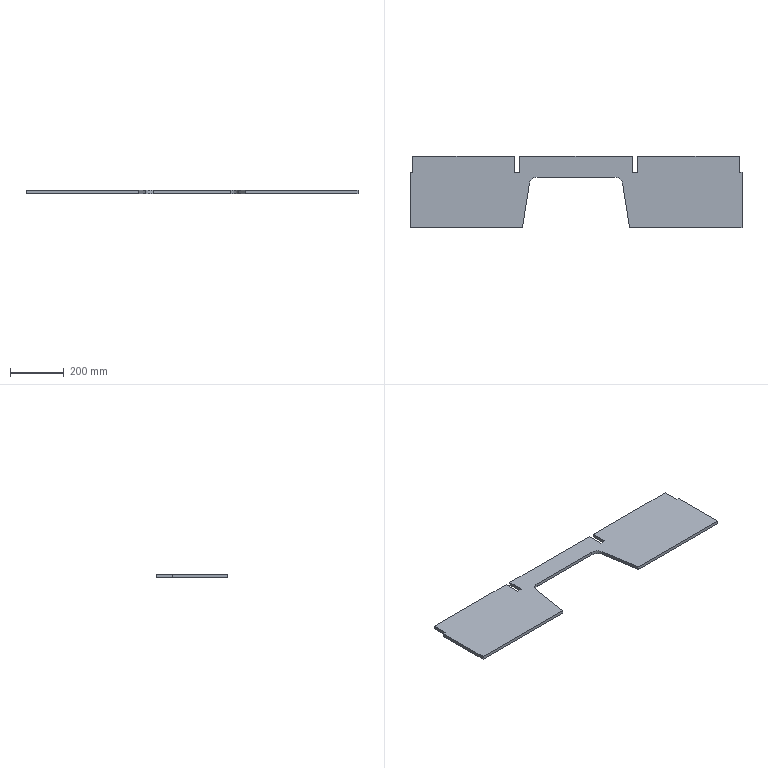Part | SolidWorks | features Extrusion 1 | 1 solid | 24 faces | box 1240 x 268 x 12 mm | volume 3104432 mm3 | plane 22 | cylinder 2 | commonest cylinder face diameters 60 x2
STEP:
#1=CARTESIAN_POINT('',(0.,208.,0.));
#2=VERTEX_POINT('',#1);
#3=CARTESIAN_POINT('',(0.,0.,0.));
#4=VERTEX_POINT('',#3);
#5=CARTESIAN_POINT('',(0.,0.,0.));
#6=DIRECTION('',(0.,-1.,0.));
#7=VECTOR('',#6,1000.);
#8=LINE('',#5,#7);
#9=EDGE_CURVE('',#2,#4,#8,.T.);
#10=ORIENTED_EDGE('',*,*,#9,.T.);
#11=CARTESIAN_POINT('',(0.,0.,12.));
#12=VERTEX_POINT('',#11);
#13=CARTESIAN_POINT('',(0.,0.,12.));
#14=DIRECTION('',(0.,0.,-1.));
#15=VECTOR('',#14,1000.);
#16=LINE('',#13,#15);
#17=EDGE_CURVE('',#12,#4,#16,.T.);
#18=ORIENTED_EDGE('',*,*,#17,.F.);
#19=CARTESIAN_POINT('',(0.,208.,12.));
#20=VERTEX_POINT('',#19);
#21=CARTESIAN_POINT('',(0.,0.,12.));
#22=DIRECTION('',(0.,-1.,0.));
#23=VECTOR('',#22,1000.);
#24=LINE('',#21,#23);
#25=EDGE_CURVE('',#20,#12,#24,.T.);
#26=ORIENTED_EDGE('',*,*,#25,.F.);
#27=CARTESIAN_POINT('',(0.,208.,12.));
#28=DIRECTION('',(0.,0.,-1.));
#29=VECTOR('',#28,1000.);
#30=LINE('',#27,#29);
#31=EDGE_CURVE('',#20,#2,#30,.T.);
#32=ORIENTED_EDGE('',*,*,#31,.T.);
#33=EDGE_LOOP('',(#10,#18,#26,#32));
#34=FACE_OUTER_BOUND('',#33,.T.);
#35=CARTESIAN_POINT('',(0.,0.,12.));
#36=DIRECTION('',(1.,0.,0.));
#37=DIRECTION('',(0.,0.,-1.));
#38=AXIS2_PLACEMENT_3D('',#35,#36,#37);
#39=PLANE('',#38);
#40=ADVANCED_FACE('',(#34),#39,.F.);
#41=CARTESIAN_POINT('',(420.,0.,0.));
#42=VERTEX_POINT('',#41);
#43=CARTESIAN_POINT('',(0.,0.,0.));
#44=DIRECTION('',(1.,0.,0.));
#45=VECTOR('',#44,1000.);
#46=LINE('',#43,#45);
#47=EDGE_CURVE('',#4,#42,#46,.T.);
#48=ORIENTED_EDGE('',*,*,#47,.T.);
#49=CARTESIAN_POINT('',(420.,0.,12.));
#50=VERTEX_POINT('',#49);
#51=CARTESIAN_POINT('',(420.,0.,12.));
#52=DIRECTION('',(0.,0.,-1.));
#53=VECTOR('',#52,1000.);
#54=LINE('',#51,#53);
#55=EDGE_CURVE('',#50,#42,#54,.T.);
#56=ORIENTED_EDGE('',*,*,#55,.F.);
#57=CARTESIAN_POINT('',(0.,0.,12.));
#58=DIRECTION('',(1.,0.,0.));
#59=VECTOR('',#58,1000.);
#60=LINE('',#57,#59);
#61=EDGE_CURVE('',#12,#50,#60,.T.);
#62=ORIENTED_EDGE('',*,*,#61,.F.);
#63=ORIENTED_EDGE('',*,*,#17,.T.);
#64=EDGE_LOOP('',(#48,#56,#62,#63));
#65=FACE_OUTER_BOUND('',#64,.T.);
#66=CARTESIAN_POINT('',(0.,0.,12.));
#67=DIRECTION('',(0.,1.,0.));
#68=DIRECTION('',(0.,0.,1.));
#69=AXIS2_PLACEMENT_3D('',#66,#67,#68);
#70=PLANE('',#69);
#71=ADVANCED_FACE('',(#65),#70,.F.);
#72=CARTESIAN_POINT('',(446.085,164.693,0.));
#73=VERTEX_POINT('',#72);
#74=CARTESIAN_POINT('',(420.,0.,0.));
#75=DIRECTION('',(0.1564,0.9877,0.));
#76=VECTOR('',#75,1000.);
#77=LINE('',#74,#76);
#78=EDGE_CURVE('',#42,#73,#77,.T.);
#79=ORIENTED_EDGE('',*,*,#78,.T.);
#80=CARTESIAN_POINT('',(446.085,164.693,12.));
#81=VERTEX_POINT('',#80);
#82=CARTESIAN_POINT('',(446.085,164.693,12.));
#83=DIRECTION('',(0.,0.,-1.));
#84=VECTOR('',#83,1000.);
#85=LINE('',#82,#84);
#86=EDGE_CURVE('',#81,#73,#85,.T.);
#87=ORIENTED_EDGE('',*,*,#86,.F.);
#88=CARTESIAN_POINT('',(420.,0.,12.));
#89=DIRECTION('',(0.1564,0.9877,0.));
#90=VECTOR('',#89,1000.);
#91=LINE('',#88,#90);
#92=EDGE_CURVE('',#50,#81,#91,.T.);
#93=ORIENTED_EDGE('',*,*,#92,.F.);
#94=ORIENTED_EDGE('',*,*,#55,.T.);
#95=EDGE_LOOP('',(#79,#87,#93,#94));
#96=FACE_OUTER_BOUND('',#95,.T.);
#97=CARTESIAN_POINT('',(420.,0.,12.));
#98=DIRECTION('',(-0.9877,0.1564,0.));
#99=DIRECTION('',(-0.1564,-0.9877,0.));
#100=AXIS2_PLACEMENT_3D('',#97,#98,#99);
#101=PLANE('',#100);
#102=ADVANCED_FACE('',(#96),#101,.F.);
#103=CARTESIAN_POINT('',(475.715,190.,0.));
#104=VERTEX_POINT('',#103);
#105=CARTESIAN_POINT('',(475.715,160.,0.));
#106=DIRECTION('',(0.,0.,-1.));
#107=DIRECTION('',(-1.,0.,0.));
#108=AXIS2_PLACEMENT_3D('',#105,#106,#107);
#109=CIRCLE('',#108,30.);
#110=EDGE_CURVE('',#73,#104,#109,.T.);
#111=ORIENTED_EDGE('',*,*,#110,.T.);
#112=CARTESIAN_POINT('',(475.715,190.,12.));
#113=VERTEX_POINT('',#112);
#114=CARTESIAN_POINT('',(475.715,190.,12.));
#115=DIRECTION('',(0.,0.,-1.));
#116=VECTOR('',#115,1000.);
#117=LINE('',#114,#116);
#118=EDGE_CURVE('',#113,#104,#117,.T.);
#119=ORIENTED_EDGE('',*,*,#118,.F.);
#120=CARTESIAN_POINT('',(475.715,160.,12.));
#121=DIRECTION('',(0.,0.,-1.));
#122=DIRECTION('',(-1.,0.,0.));
#123=AXIS2_PLACEMENT_3D('',#120,#121,#122);
#124=CIRCLE('',#123,30.);
#125=EDGE_CURVE('',#81,#113,#124,.T.);
#126=ORIENTED_EDGE('',*,*,#125,.F.);
#127=ORIENTED_EDGE('',*,*,#86,.T.);
#128=EDGE_LOOP('',(#111,#119,#126,#127));
#129=FACE_OUTER_BOUND('',#128,.T.);
#130=CARTESIAN_POINT('',(475.715,160.,12.));
#131=DIRECTION('',(0.,0.,-1.));
#132=DIRECTION('',(-1.,0.,0.));
#133=AXIS2_PLACEMENT_3D('',#130,#131,#132);
#134=CYLINDRICAL_SURFACE('',#133,30.);
#135=ADVANCED_FACE('',(#129),#134,.F.);
#136=CARTESIAN_POINT('',(764.285,190.,0.));
#137=VERTEX_POINT('',#136);
#138=CARTESIAN_POINT('',(475.715,190.,0.));
#139=DIRECTION('',(1.,0.,0.));
#140=VECTOR('',#139,1000.);
#141=LINE('',#138,#140);
#142=EDGE_CURVE('',#104,#137,#141,.T.);
#143=ORIENTED_EDGE('',*,*,#142,.T.);
#144=CARTESIAN_POINT('',(764.285,190.,12.));
#145=VERTEX_POINT('',#144);
#146=CARTESIAN_POINT('',(764.285,190.,12.));
#147=DIRECTION('',(0.,0.,-1.));
#148=VECTOR('',#147,1000.);
#149=LINE('',#146,#148);
#150=EDGE_CURVE('',#145,#137,#149,.T.);
#151=ORIENTED_EDGE('',*,*,#150,.F.);
#152=CARTESIAN_POINT('',(475.715,190.,12.));
#153=DIRECTION('',(1.,0.,0.));
#154=VECTOR('',#153,1000.);
#155=LINE('',#152,#154);
#156=EDGE_CURVE('',#113,#145,#155,.T.);
#157=ORIENTED_EDGE('',*,*,#156,.F.);
#158=ORIENTED_EDGE('',*,*,#118,.T.);
#159=EDGE_LOOP('',(#143,#151,#157,#158));
#160=FACE_OUTER_BOUND('',#159,.T.);
#161=CARTESIAN_POINT('',(475.715,190.,12.));
#162=DIRECTION('',(0.,1.,0.));
#163=DIRECTION('',(-1.,0.,0.));
#164=AXIS2_PLACEMENT_3D('',#161,#162,#163);
#165=PLANE('',#164);
#166=ADVANCED_FACE('',(#160),#165,.F.);
#167=CARTESIAN_POINT('',(793.915,164.693,0.));
#168=VERTEX_POINT('',#167);
#169=CARTESIAN_POINT('',(764.285,160.,0.));
#170=DIRECTION('',(0.,0.,-1.));
#171=DIRECTION('',(1.,0.,0.));
#172=AXIS2_PLACEMENT_3D('',#169,#170,#171);
#173=CIRCLE('',#172,30.);
#174=EDGE_CURVE('',#137,#168,#173,.T.);
#175=ORIENTED_EDGE('',*,*,#174,.T.);
#176=CARTESIAN_POINT('',(793.915,164.693,12.));
#177=VERTEX_POINT('',#176);
#178=CARTESIAN_POINT('',(793.915,164.693,12.));
#179=DIRECTION('',(0.,0.,-1.));
#180=VECTOR('',#179,1000.);
#181=LINE('',#178,#180);
#182=EDGE_CURVE('',#177,#168,#181,.T.);
#183=ORIENTED_EDGE('',*,*,#182,.F.);
#184=CARTESIAN_POINT('',(764.285,160.,12.));
#185=DIRECTION('',(0.,0.,-1.));
#186=DIRECTION('',(1.,0.,0.));
#187=AXIS2_PLACEMENT_3D('',#184,#185,#186);
#188=CIRCLE('',#187,30.);
#189=EDGE_CURVE('',#145,#177,#188,.T.);
#190=ORIENTED_EDGE('',*,*,#189,.F.);
#191=ORIENTED_EDGE('',*,*,#150,.T.);
#192=EDGE_LOOP('',(#175,#183,#190,#191));
#193=FACE_OUTER_BOUND('',#192,.T.);
#194=CARTESIAN_POINT('',(764.285,160.,12.));
#195=DIRECTION('',(0.,0.,-1.));
#196=DIRECTION('',(-1.,0.,0.));
#197=AXIS2_PLACEMENT_3D('',#194,#195,#196);
#198=CYLINDRICAL_SURFACE('',#197,30.);
#199=ADVANCED_FACE('',(#193),#198,.F.);
#200=CARTESIAN_POINT('',(820.,0.,0.));
#201=VERTEX_POINT('',#200);
#202=CARTESIAN_POINT('',(820.,0.,0.));
#203=DIRECTION('',(0.1564,-0.9877,0.));
#204=VECTOR('',#203,1000.);
#205=LINE('',#202,#204);
#206=EDGE_CURVE('',#168,#201,#205,.T.);
#207=ORIENTED_EDGE('',*,*,#206,.T.);
#208=CARTESIAN_POINT('',(820.,0.,12.));
#209=VERTEX_POINT('',#208);
#210=CARTESIAN_POINT('',(820.,0.,12.));
#211=DIRECTION('',(0.,0.,-1.));
#212=VECTOR('',#211,1000.);
#213=LINE('',#210,#212);
#214=EDGE_CURVE('',#209,#201,#213,.T.);
#215=ORIENTED_EDGE('',*,*,#214,.F.);
#216=CARTESIAN_POINT('',(820.,0.,12.));
#217=DIRECTION('',(0.1564,-0.9877,0.));
#218=VECTOR('',#217,1000.);
#219=LINE('',#216,#218);
#220=EDGE_CURVE('',#177,#209,#219,.T.);
#221=ORIENTED_EDGE('',*,*,#220,.F.);
#222=ORIENTED_EDGE('',*,*,#182,.T.);
#223=EDGE_LOOP('',(#207,#215,#221,#222));
#224=FACE_OUTER_BOUND('',#223,.T.);
#225=CARTESIAN_POINT('',(820.,0.,12.));
#226=DIRECTION('',(0.9877,0.1564,0.));
#227=DIRECTION('',(-0.1564,0.9877,0.));
#228=AXIS2_PLACEMENT_3D('',#225,#226,#227);
#229=PLANE('',#228);
#230=ADVANCED_FACE('',(#224),#229,.F.);
#231=CARTESIAN_POINT('',(1240.,0.,0.));
#232=VERTEX_POINT('',#231);
#233=CARTESIAN_POINT('',(820.,0.,0.));
#234=DIRECTION('',(1.,0.,0.));
#235=VECTOR('',#234,1000.);
#236=LINE('',#233,#235);
#237=EDGE_CURVE('',#201,#232,#236,.T.);
#238=ORIENTED_EDGE('',*,*,#237,.T.);
#239=CARTESIAN_POINT('',(1240.,0.,12.));
#240=VERTEX_POINT('',#239);
#241=CARTESIAN_POINT('',(1240.,0.,12.));
#242=DIRECTION('',(0.,0.,-1.));
#243=VECTOR('',#242,1000.);
#244=LINE('',#241,#243);
#245=EDGE_CURVE('',#240,#232,#244,.T.);
#246=ORIENTED_EDGE('',*,*,#245,.F.);
#247=CARTESIAN_POINT('',(820.,0.,12.));
#248=DIRECTION('',(1.,0.,0.));
#249=VECTOR('',#248,1000.);
#250=LINE('',#247,#249);
#251=EDGE_CURVE('',#209,#240,#250,.T.);
#252=ORIENTED_EDGE('',*,*,#251,.F.);
#253=ORIENTED_EDGE('',*,*,#214,.T.);
#254=EDGE_LOOP('',(#238,#246,#252,#253));
#255=FACE_OUTER_BOUND('',#254,.T.);
#256=CARTESIAN_POINT('',(820.,0.,12.));
#257=DIRECTION('',(0.,1.,0.));
#258=DIRECTION('',(0.,0.,1.));
#259=AXIS2_PLACEMENT_3D('',#256,#257,#258);
#260=PLANE('',#259);
#261=ADVANCED_FACE('',(#255),#260,.F.);
#262=CARTESIAN_POINT('',(1240.,208.,0.));
#263=VERTEX_POINT('',#262);
#264=CARTESIAN_POINT('',(1240.,0.,0.));
#265=DIRECTION('',(0.,1.,0.));
#266=VECTOR('',#265,1000.);
#267=LINE('',#264,#266);
#268=EDGE_CURVE('',#232,#263,#267,.T.);
#269=ORIENTED_EDGE('',*,*,#268,.T.);
#270=CARTESIAN_POINT('',(1240.,208.,12.));
#271=VERTEX_POINT('',#270);
#272=CARTESIAN_POINT('',(1240.,208.,12.));
#273=DIRECTION('',(0.,0.,-1.));
#274=VECTOR('',#273,1000.);
#275=LINE('',#272,#274);
#276=EDGE_CURVE('',#271,#263,#275,.T.);
#277=ORIENTED_EDGE('',*,*,#276,.F.);
#278=CARTESIAN_POINT('',(1240.,0.,12.));
#279=DIRECTION('',(0.,1.,0.));
#280=VECTOR('',#279,1000.);
#281=LINE('',#278,#280);
#282=EDGE_CURVE('',#240,#271,#281,.T.);
#283=ORIENTED_EDGE('',*,*,#282,.F.);
#284=ORIENTED_EDGE('',*,*,#245,.T.);
#285=EDGE_LOOP('',(#269,#277,#283,#284));
#286=FACE_OUTER_BOUND('',#285,.T.);
#287=CARTESIAN_POINT('',(1240.,0.,12.));
#288=DIRECTION('',(-1.,0.,0.));
#289=DIRECTION('',(0.,0.,1.));
#290=AXIS2_PLACEMENT_3D('',#287,#288,#289);
#291=PLANE('',#290);
#292=ADVANCED_FACE('',(#286),#291,.F.);
#293=CARTESIAN_POINT('',(1230.,208.,0.));
#294=VERTEX_POINT('',#293);
#295=CARTESIAN_POINT('',(1230.,208.,0.));
#296=DIRECTION('',(-1.,0.,0.));
#297=VECTOR('',#296,1000.);
#298=LINE('',#295,#297);
#299=EDGE_CURVE('',#263,#294,#298,.T.);
#300=ORIENTED_EDGE('',*,*,#299,.T.);
#301=CARTESIAN_POINT('',(1230.,208.,12.));
#302=VERTEX_POINT('',#301);
#303=CARTESIAN_POINT('',(1230.,208.,12.));
#304=DIRECTION('',(0.,0.,-1.));
#305=VECTOR('',#304,1000.);
#306=LINE('',#303,#305);
#307=EDGE_CURVE('',#302,#294,#306,.T.);
#308=ORIENTED_EDGE('',*,*,#307,.F.);
#309=CARTESIAN_POINT('',(1230.,208.,12.));
#310=DIRECTION('',(-1.,0.,0.));
#311=VECTOR('',#310,1000.);
#312=LINE('',#309,#311);
#313=EDGE_CURVE('',#271,#302,#312,.T.);
#314=ORIENTED_EDGE('',*,*,#313,.F.);
#315=ORIENTED_EDGE('',*,*,#276,.T.);
#316=EDGE_LOOP('',(#300,#308,#314,#315));
#317=FACE_OUTER_BOUND('',#316,.T.);
#318=CARTESIAN_POINT('',(1230.,208.,12.));
#319=DIRECTION('',(0.,-1.,0.));
#320=DIRECTION('',(0.,0.,-1.));
#321=AXIS2_PLACEMENT_3D('',#318,#319,#320);
#322=PLANE('',#321);
#323=ADVANCED_FACE('',(#317),#322,.F.);
#324=CARTESIAN_POINT('',(1230.,268.,0.));
#325=VERTEX_POINT('',#324);
#326=CARTESIAN_POINT('',(1230.,268.,0.));
#327=DIRECTION('',(0.,1.,0.));
#328=VECTOR('',#327,1000.);
#329=LINE('',#326,#328);
#330=EDGE_CURVE('',#294,#325,#329,.T.);
#331=ORIENTED_EDGE('',*,*,#330,.T.);
#332=CARTESIAN_POINT('',(1230.,268.,12.));
#333=VERTEX_POINT('',#332);
#334=CARTESIAN_POINT('',(1230.,268.,12.));
#335=DIRECTION('',(0.,0.,-1.));
#336=VECTOR('',#335,1000.);
#337=LINE('',#334,#336);
#338=EDGE_CURVE('',#333,#325,#337,.T.);
#339=ORIENTED_EDGE('',*,*,#338,.F.);
#340=CARTESIAN_POINT('',(1230.,268.,12.));
#341=DIRECTION('',(0.,1.,0.));
#342=VECTOR('',#341,1000.);
#343=LINE('',#340,#342);
#344=EDGE_CURVE('',#302,#333,#343,.T.);
#345=ORIENTED_EDGE('',*,*,#344,.F.);
#346=ORIENTED_EDGE('',*,*,#307,.T.);
#347=EDGE_LOOP('',(#331,#339,#345,#346));
#348=FACE_OUTER_BOUND('',#347,.T.);
#349=CARTESIAN_POINT('',(1230.,268.,12.));
#350=DIRECTION('',(-1.,0.,0.));
#351=DIRECTION('',(0.,0.,1.));
#352=AXIS2_PLACEMENT_3D('',#349,#350,#351);
#353=PLANE('',#352);
#354=ADVANCED_FACE('',(#348),#353,.F.);
#355=CARTESIAN_POINT('',(850.,268.,0.));
#356=VERTEX_POINT('',#355);
#357=CARTESIAN_POINT('',(850.,268.,0.));
#358=DIRECTION('',(-1.,0.,0.));
#359=VECTOR('',#358,1000.);
#360=LINE('',#357,#359);
#361=EDGE_CURVE('',#325,#356,#360,.T.);
#362=ORIENTED_EDGE('',*,*,#361,.T.);
#363=CARTESIAN_POINT('',(850.,268.,12.));
#364=VERTEX_POINT('',#363);
#365=CARTESIAN_POINT('',(850.,268.,12.));
#366=DIRECTION('',(0.,0.,-1.));
#367=VECTOR('',#366,1000.);
#368=LINE('',#365,#367);
#369=EDGE_CURVE('',#364,#356,#368,.T.);
#370=ORIENTED_EDGE('',*,*,#369,.F.);
#371=CARTESIAN_POINT('',(850.,268.,12.));
#372=DIRECTION('',(-1.,0.,0.));
#373=VECTOR('',#372,1000.);
#374=LINE('',#371,#373);
#375=EDGE_CURVE('',#333,#364,#374,.T.);
#376=ORIENTED_EDGE('',*,*,#375,.F.);
#377=ORIENTED_EDGE('',*,*,#338,.T.);
#378=EDGE_LOOP('',(#362,#370,#376,#377));
#379=FACE_OUTER_BOUND('',#378,.T.);
#380=CARTESIAN_POINT('',(850.,268.,12.));
#381=DIRECTION('',(0.,-1.,0.));
#382=DIRECTION('',(0.,0.,-1.));
#383=AXIS2_PLACEMENT_3D('',#380,#381,#382);
#384=PLANE('',#383);
#385=ADVANCED_FACE('',(#379),#384,.F.);
#386=CARTESIAN_POINT('',(850.,208.,0.));
#387=VERTEX_POINT('',#386);
#388=CARTESIAN_POINT('',(850.,268.,0.));
#389=DIRECTION('',(0.,-1.,0.));
#390=VECTOR('',#389,1000.);
#391=LINE('',#388,#390);
#392=EDGE_CURVE('',#356,#387,#391,.T.);
#393=ORIENTED_EDGE('',*,*,#392,.T.);
#394=CARTESIAN_POINT('',(850.,208.,12.));
#395=VERTEX_POINT('',#394);
#396=CARTESIAN_POINT('',(850.,208.,12.));
#397=DIRECTION('',(0.,0.,-1.));
#398=VECTOR('',#397,1000.);
#399=LINE('',#396,#398);
#400=EDGE_CURVE('',#395,#387,#399,.T.);
#401=ORIENTED_EDGE('',*,*,#400,.F.);
#402=CARTESIAN_POINT('',(850.,268.,12.));
#403=DIRECTION('',(0.,-1.,0.));
#404=VECTOR('',#403,1000.);
#405=LINE('',#402,#404);
#406=EDGE_CURVE('',#364,#395,#405,.T.);
#407=ORIENTED_EDGE('',*,*,#406,.F.);
#408=ORIENTED_EDGE('',*,*,#369,.T.);
#409=EDGE_LOOP('',(#393,#401,#407,#408));
#410=FACE_OUTER_BOUND('',#409,.T.);
#411=CARTESIAN_POINT('',(850.,268.,12.));
#412=DIRECTION('',(1.,0.,0.));
#413=DIRECTION('',(0.,0.,-1.));
#414=AXIS2_PLACEMENT_3D('',#411,#412,#413);
#415=PLANE('',#414);
#416=ADVANCED_FACE('',(#410),#415,.F.);
#417=CARTESIAN_POINT('',(830.,208.,0.));
#418=VERTEX_POINT('',#417);
#419=CARTESIAN_POINT('',(830.,208.,0.));
#420=DIRECTION('',(-1.,0.,0.));
#421=VECTOR('',#420,1000.);
#422=LINE('',#419,#421);
#423=EDGE_CURVE('',#387,#418,#422,.T.);
#424=ORIENTED_EDGE('',*,*,#423,.T.);
#425=CARTESIAN_POINT('',(830.,208.,12.));
#426=VERTEX_POINT('',#425);
#427=CARTESIAN_POINT('',(830.,208.,12.));
#428=DIRECTION('',(0.,0.,-1.));
#429=VECTOR('',#428,1000.);
#430=LINE('',#427,#429);
#431=EDGE_CURVE('',#426,#418,#430,.T.);
#432=ORIENTED_EDGE('',*,*,#431,.F.);
#433=CARTESIAN_POINT('',(830.,208.,12.));
#434=DIRECTION('',(-1.,0.,0.));
#435=VECTOR('',#434,1000.);
#436=LINE('',#433,#435);
#437=EDGE_CURVE('',#395,#426,#436,.T.);
#438=ORIENTED_EDGE('',*,*,#437,.F.);
#439=ORIENTED_EDGE('',*,*,#400,.T.);
#440=EDGE_LOOP('',(#424,#432,#438,#439));
#441=FACE_OUTER_BOUND('',#440,.T.);
#442=CARTESIAN_POINT('',(830.,208.,12.));
#443=DIRECTION('',(0.,-1.,0.));
#444=DIRECTION('',(0.,0.,-1.));
#445=AXIS2_PLACEMENT_3D('',#442,#443,#444);
#446=PLANE('',#445);
#447=ADVANCED_FACE('',(#441),#446,.F.);
#448=CARTESIAN_POINT('',(830.,268.,0.));
#449=VERTEX_POINT('',#448);
#450=CARTESIAN_POINT('',(830.,268.,0.));
#451=DIRECTION('',(0.,1.,0.));
#452=VECTOR('',#451,1000.);
#453=LINE('',#450,#452);
#454=EDGE_CURVE('',#418,#449,#453,.T.);
#455=ORIENTED_EDGE('',*,*,#454,.T.);
#456=CARTESIAN_POINT('',(830.,268.,12.));
#457=VERTEX_POINT('',#456);
#458=CARTESIAN_POINT('',(830.,268.,12.));
#459=DIRECTION('',(0.,0.,-1.));
#460=VECTOR('',#459,1000.);
#461=LINE('',#458,#460);
#462=EDGE_CURVE('',#457,#449,#461,.T.);
#463=ORIENTED_EDGE('',*,*,#462,.F.);
#464=CARTESIAN_POINT('',(830.,268.,12.));
#465=DIRECTION('',(0.,1.,0.));
#466=VECTOR('',#465,1000.);
#467=LINE('',#464,#466);
#468=EDGE_CURVE('',#426,#457,#467,.T.);
#469=ORIENTED_EDGE('',*,*,#468,.F.);
#470=ORIENTED_EDGE('',*,*,#431,.T.);
#471=EDGE_LOOP('',(#455,#463,#469,#470));
#472=FACE_OUTER_BOUND('',#471,.T.);
#473=CARTESIAN_POINT('',(830.,268.,12.));
#474=DIRECTION('',(-1.,0.,0.));
#475=DIRECTION('',(0.,0.,1.));
#476=AXIS2_PLACEMENT_3D('',#473,#474,#475);
#477=PLANE('',#476);
#478=ADVANCED_FACE('',(#472),#477,.F.);
#479=CARTESIAN_POINT('',(410.,268.,0.));
#480=VERTEX_POINT('',#479);
#481=CARTESIAN_POINT('',(410.,268.,0.));
#482=DIRECTION('',(-1.,0.,0.));
#483=VECTOR('',#482,1000.);
#484=LINE('',#481,#483);
#485=EDGE_CURVE('',#449,#480,#484,.T.);
#486=ORIENTED_EDGE('',*,*,#485,.T.);
#487=CARTESIAN_POINT('',(410.,268.,12.));
#488=VERTEX_POINT('',#487);
#489=CARTESIAN_POINT('',(410.,268.,12.));
#490=DIRECTION('',(0.,0.,-1.));
#491=VECTOR('',#490,1000.);
#492=LINE('',#489,#491);
#493=EDGE_CURVE('',#488,#480,#492,.T.);
#494=ORIENTED_EDGE('',*,*,#493,.F.);
#495=CARTESIAN_POINT('',(410.,268.,12.));
#496=DIRECTION('',(-1.,0.,0.));
#497=VECTOR('',#496,1000.);
#498=LINE('',#495,#497);
#499=EDGE_CURVE('',#457,#488,#498,.T.);
#500=ORIENTED_EDGE('',*,*,#499,.F.);
#501=ORIENTED_EDGE('',*,*,#462,.T.);
#502=EDGE_LOOP('',(#486,#494,#500,#501));
#503=FACE_OUTER_BOUND('',#502,.T.);
#504=CARTESIAN_POINT('',(410.,268.,12.));
#505=DIRECTION('',(0.,-1.,0.));
#506=DIRECTION('',(0.,0.,-1.));
#507=AXIS2_PLACEMENT_3D('',#504,#505,#506);
#508=PLANE('',#507);
#509=ADVANCED_FACE('',(#503),#508,.F.);
#510=CARTESIAN_POINT('',(410.,208.,0.));
#511=VERTEX_POINT('',#510);
#512=CARTESIAN_POINT('',(410.,268.,0.));
#513=DIRECTION('',(0.,-1.,0.));
#514=VECTOR('',#513,1000.);
#515=LINE('',#512,#514);
#516=EDGE_CURVE('',#480,#511,#515,.T.);
#517=ORIENTED_EDGE('',*,*,#516,.T.);
#518=CARTESIAN_POINT('',(410.,208.,12.));
#519=VERTEX_POINT('',#518);
#520=CARTESIAN_POINT('',(410.,208.,12.));
#521=DIRECTION('',(0.,0.,-1.));
#522=VECTOR('',#521,1000.);
#523=LINE('',#520,#522);
#524=EDGE_CURVE('',#519,#511,#523,.T.);
#525=ORIENTED_EDGE('',*,*,#524,.F.);
#526=CARTESIAN_POINT('',(410.,268.,12.));
#527=DIRECTION('',(0.,-1.,0.));
#528=VECTOR('',#527,1000.);
#529=LINE('',#526,#528);
#530=EDGE_CURVE('',#488,#519,#529,.T.);
#531=ORIENTED_EDGE('',*,*,#530,.F.);
#532=ORIENTED_EDGE('',*,*,#493,.T.);
#533=EDGE_LOOP('',(#517,#525,#531,#532));
#534=FACE_OUTER_BOUND('',#533,.T.);
#535=CARTESIAN_POINT('',(410.,268.,12.));
#536=DIRECTION('',(1.,0.,0.));
#537=DIRECTION('',(0.,0.,-1.));
#538=AXIS2_PLACEMENT_3D('',#535,#536,#537);
#539=PLANE('',#538);
#540=ADVANCED_FACE('',(#534),#539,.F.);
#541=CARTESIAN_POINT('',(390.,208.,0.));
#542=VERTEX_POINT('',#541);
#543=CARTESIAN_POINT('',(390.,208.,0.));
#544=DIRECTION('',(-1.,0.,0.));
#545=VECTOR('',#544,1000.);
#546=LINE('',#543,#545);
#547=EDGE_CURVE('',#511,#542,#546,.T.);
#548=ORIENTED_EDGE('',*,*,#547,.T.);
#549=CARTESIAN_POINT('',(390.,208.,12.));
#550=VERTEX_POINT('',#549);
#551=CARTESIAN_POINT('',(390.,208.,12.));
#552=DIRECTION('',(0.,0.,-1.));
#553=VECTOR('',#552,1000.);
#554=LINE('',#551,#553);
#555=EDGE_CURVE('',#550,#542,#554,.T.);
#556=ORIENTED_EDGE('',*,*,#555,.F.);
#557=CARTESIAN_POINT('',(390.,208.,12.));
#558=DIRECTION('',(-1.,0.,0.));
#559=VECTOR('',#558,1000.);
#560=LINE('',#557,#559);
#561=EDGE_CURVE('',#519,#550,#560,.T.);
#562=ORIENTED_EDGE('',*,*,#561,.F.);
#563=ORIENTED_EDGE('',*,*,#524,.T.);
#564=EDGE_LOOP('',(#548,#556,#562,#563));
#565=FACE_OUTER_BOUND('',#564,.T.);
#566=CARTESIAN_POINT('',(390.,208.,12.));
#567=DIRECTION('',(0.,-1.,0.));
#568=DIRECTION('',(0.,0.,-1.));
#569=AXIS2_PLACEMENT_3D('',#566,#567,#568);
#570=PLANE('',#569);
#571=ADVANCED_FACE('',(#565),#570,.F.);
#572=CARTESIAN_POINT('',(390.,268.,0.));
#573=VERTEX_POINT('',#572);
#574=CARTESIAN_POINT('',(390.,268.,0.));
#575=DIRECTION('',(0.,1.,0.));
#576=VECTOR('',#575,1000.);
#577=LINE('',#574,#576);
#578=EDGE_CURVE('',#542,#573,#577,.T.);
#579=ORIENTED_EDGE('',*,*,#578,.T.);
#580=CARTESIAN_POINT('',(390.,268.,12.));
#581=VERTEX_POINT('',#580);
#582=CARTESIAN_POINT('',(390.,268.,12.));
#583=DIRECTION('',(0.,0.,-1.));
#584=VECTOR('',#583,1000.);
#585=LINE('',#582,#584);
#586=EDGE_CURVE('',#581,#573,#585,.T.);
#587=ORIENTED_EDGE('',*,*,#586,.F.);
#588=CARTESIAN_POINT('',(390.,268.,12.));
#589=DIRECTION('',(0.,1.,0.));
#590=VECTOR('',#589,1000.);
#591=LINE('',#588,#590);
#592=EDGE_CURVE('',#550,#581,#591,.T.);
#593=ORIENTED_EDGE('',*,*,#592,.F.);
#594=ORIENTED_EDGE('',*,*,#555,.T.);
#595=EDGE_LOOP('',(#579,#587,#593,#594));
#596=FACE_OUTER_BOUND('',#595,.T.);
#597=CARTESIAN_POINT('',(390.,268.,12.));
#598=DIRECTION('',(-1.,0.,0.));
#599=DIRECTION('',(0.,0.,1.));
#600=AXIS2_PLACEMENT_3D('',#597,#598,#599);
#601=PLANE('',#600);
#602=ADVANCED_FACE('',(#596),#601,.F.);
#603=CARTESIAN_POINT('',(10.,268.,0.));
#604=VERTEX_POINT('',#603);
#605=CARTESIAN_POINT('',(10.,268.,0.));
#606=DIRECTION('',(-1.,0.,0.));
#607=VECTOR('',#606,1000.);
#608=LINE('',#605,#607);
#609=EDGE_CURVE('',#573,#604,#608,.T.);
#610=ORIENTED_EDGE('',*,*,#609,.T.);
#611=CARTESIAN_POINT('',(10.,268.,12.));
#612=VERTEX_POINT('',#611);
#613=CARTESIAN_POINT('',(10.,268.,12.));
#614=DIRECTION('',(0.,0.,-1.));
#615=VECTOR('',#614,1000.);
#616=LINE('',#613,#615);
#617=EDGE_CURVE('',#612,#604,#616,.T.);
#618=ORIENTED_EDGE('',*,*,#617,.F.);
#619=CARTESIAN_POINT('',(10.,268.,12.));
#620=DIRECTION('',(-1.,0.,0.));
#621=VECTOR('',#620,1000.);
#622=LINE('',#619,#621);
#623=EDGE_CURVE('',#581,#612,#622,.T.);
#624=ORIENTED_EDGE('',*,*,#623,.F.);
#625=ORIENTED_EDGE('',*,*,#586,.T.);
#626=EDGE_LOOP('',(#610,#618,#624,#625));
#627=FACE_OUTER_BOUND('',#626,.T.);
#628=CARTESIAN_POINT('',(10.,268.,12.));
#629=DIRECTION('',(0.,-1.,0.));
#630=DIRECTION('',(0.,0.,-1.));
#631=AXIS2_PLACEMENT_3D('',#628,#629,#630);
#632=PLANE('',#631);
#633=ADVANCED_FACE('',(#627),#632,.F.);
#634=CARTESIAN_POINT('',(10.,208.,0.));
#635=VERTEX_POINT('',#634);
#636=CARTESIAN_POINT('',(10.,268.,0.));
#637=DIRECTION('',(0.,-1.,0.));
#638=VECTOR('',#637,1000.);
#639=LINE('',#636,#638);
#640=EDGE_CURVE('',#604,#635,#639,.T.);
#641=ORIENTED_EDGE('',*,*,#640,.T.);
#642=CARTESIAN_POINT('',(10.,208.,12.));
#643=VERTEX_POINT('',#642);
#644=CARTESIAN_POINT('',(10.,208.,12.));
#645=DIRECTION('',(0.,0.,-1.));
#646=VECTOR('',#645,1000.);
#647=LINE('',#644,#646);
#648=EDGE_CURVE('',#643,#635,#647,.T.);
#649=ORIENTED_EDGE('',*,*,#648,.F.);
#650=CARTESIAN_POINT('',(10.,268.,12.));
#651=DIRECTION('',(0.,-1.,0.));
#652=VECTOR('',#651,1000.);
#653=LINE('',#650,#652);
#654=EDGE_CURVE('',#612,#643,#653,.T.);
#655=ORIENTED_EDGE('',*,*,#654,.F.);
#656=ORIENTED_EDGE('',*,*,#617,.T.);
#657=EDGE_LOOP('',(#641,#649,#655,#656));
#658=FACE_OUTER_BOUND('',#657,.T.);
#659=CARTESIAN_POINT('',(10.,268.,12.));
#660=DIRECTION('',(1.,0.,0.));
#661=DIRECTION('',(0.,1.,0.));
#662=AXIS2_PLACEMENT_3D('',#659,#660,#661);
#663=PLANE('',#662);
#664=ADVANCED_FACE('',(#658),#663,.F.);
#665=CARTESIAN_POINT('',(0.,208.,0.));
#666=DIRECTION('',(-1.,0.,0.));
#667=VECTOR('',#666,1000.);
#668=LINE('',#665,#667);
#669=EDGE_CURVE('',#635,#2,#668,.T.);
#670=ORIENTED_EDGE('',*,*,#669,.T.);
#671=ORIENTED_EDGE('',*,*,#31,.F.);
#672=CARTESIAN_POINT('',(0.,208.,12.));
#673=DIRECTION('',(-1.,0.,0.));
#674=VECTOR('',#673,1000.);
#675=LINE('',#672,#674);
#676=EDGE_CURVE('',#643,#20,#675,.T.);
#677=ORIENTED_EDGE('',*,*,#676,.F.);
#678=ORIENTED_EDGE('',*,*,#648,.T.);
#679=EDGE_LOOP('',(#670,#671,#677,#678));
#680=FACE_OUTER_BOUND('',#679,.T.);
#681=CARTESIAN_POINT('',(0.,208.,12.));
#682=DIRECTION('',(0.,-1.,0.));
#683=DIRECTION('',(0.,0.,-1.));
#684=AXIS2_PLACEMENT_3D('',#681,#682,#683);
#685=PLANE('',#684);
#686=ADVANCED_FACE('',(#680),#685,.F.);
#687=ORIENTED_EDGE('',*,*,#25,.T.);
#688=ORIENTED_EDGE('',*,*,#61,.T.);
#689=ORIENTED_EDGE('',*,*,#92,.T.);
#690=ORIENTED_EDGE('',*,*,#125,.T.);
#691=ORIENTED_EDGE('',*,*,#156,.T.);
#692=ORIENTED_EDGE('',*,*,#189,.T.);
#693=ORIENTED_EDGE('',*,*,#220,.T.);
#694=ORIENTED_EDGE('',*,*,#251,.T.);
#695=ORIENTED_EDGE('',*,*,#282,.T.);
#696=ORIENTED_EDGE('',*,*,#313,.T.);
#697=ORIENTED_EDGE('',*,*,#344,.T.);
#698=ORIENTED_EDGE('',*,*,#375,.T.);
#699=ORIENTED_EDGE('',*,*,#406,.T.);
#700=ORIENTED_EDGE('',*,*,#437,.T.);
#701=ORIENTED_EDGE('',*,*,#468,.T.);
#702=ORIENTED_EDGE('',*,*,#499,.T.);
#703=ORIENTED_EDGE('',*,*,#530,.T.);
#704=ORIENTED_EDGE('',*,*,#561,.T.);
#705=ORIENTED_EDGE('',*,*,#592,.T.);
#706=ORIENTED_EDGE('',*,*,#623,.T.);
#707=ORIENTED_EDGE('',*,*,#654,.T.);
#708=ORIENTED_EDGE('',*,*,#676,.T.);
#709=EDGE_LOOP('',(#687,#688,#689,#690,#691,#692,#693,#694,#695,#696,#697,#698,#699,#700,#701,#702,#703,#704,#705,#706,#707,#708));
#710=FACE_OUTER_BOUND('',#709,.T.);
#711=CARTESIAN_POINT('',(764.285,160.,12.));
#712=DIRECTION('',(0.,0.,1.));
#713=DIRECTION('',(1.,0.,0.));
#714=AXIS2_PLACEMENT_3D('',#711,#712,#713);
#715=PLANE('',#714);
#716=ADVANCED_FACE('',(#710),#715,.T.);
#717=ORIENTED_EDGE('',*,*,#9,.F.);
#718=ORIENTED_EDGE('',*,*,#669,.F.);
#719=ORIENTED_EDGE('',*,*,#640,.F.);
#720=ORIENTED_EDGE('',*,*,#609,.F.);
#721=ORIENTED_EDGE('',*,*,#578,.F.);
#722=ORIENTED_EDGE('',*,*,#547,.F.);
#723=ORIENTED_EDGE('',*,*,#516,.F.);
#724=ORIENTED_EDGE('',*,*,#485,.F.);
#725=ORIENTED_EDGE('',*,*,#454,.F.);
#726=ORIENTED_EDGE('',*,*,#423,.F.);
#727=ORIENTED_EDGE('',*,*,#392,.F.);
#728=ORIENTED_EDGE('',*,*,#361,.F.);
#729=ORIENTED_EDGE('',*,*,#330,.F.);
#730=ORIENTED_EDGE('',*,*,#299,.F.);
#731=ORIENTED_EDGE('',*,*,#268,.F.);
#732=ORIENTED_EDGE('',*,*,#237,.F.);
#733=ORIENTED_EDGE('',*,*,#206,.F.);
#734=ORIENTED_EDGE('',*,*,#174,.F.);
#735=ORIENTED_EDGE('',*,*,#142,.F.);
#736=ORIENTED_EDGE('',*,*,#110,.F.);
#737=ORIENTED_EDGE('',*,*,#78,.F.);
#738=ORIENTED_EDGE('',*,*,#47,.F.);
#739=EDGE_LOOP('',(#717,#718,#719,#720,#721,#722,#723,#724,#725,#726,#727,#728,#729,#730,#731,#732,#733,#734,#735,#736,#737,#738));
#740=FACE_OUTER_BOUND('',#739,.T.);
#741=CARTESIAN_POINT('',(764.285,160.,0.));
#742=DIRECTION('',(0.,0.,1.));
#743=DIRECTION('',(1.,0.,0.));
#744=AXIS2_PLACEMENT_3D('',#741,#742,#743);
#745=PLANE('',#744);
#746=ADVANCED_FACE('',(#740),#745,.F.);
#747=CLOSED_SHELL('',(#40,#71,#102,#135,#166,#199,#230,#261,#292,#323,#354,#385,#416,#447,#478,#509,#540,#571,#602,#633,#664,#686,#716,#746));
#748=MANIFOLD_SOLID_BREP('',#747);
#749=CARTESIAN_POINT('',(0.,0.,0.));
#750=DIRECTION('',(0.,0.,1.));
#751=DIRECTION('',(1.,0.,0.));
#752=AXIS2_PLACEMENT_3D('',#749,#750,#751);
#753=(LENGTH_UNIT()NAMED_UNIT(*)SI_UNIT(.MILLI.,.METRE.));
#754=UNCERTAINTY_MEASURE_WITH_UNIT(LENGTH_MEASURE(0.00001),#753,'','');
#755=(NAMED_UNIT(*)PLANE_ANGLE_UNIT()SI_UNIT($,.RADIAN.));
#756=(NAMED_UNIT(*)SI_UNIT($,.STERADIAN.)SOLID_ANGLE_UNIT());
#757=(GEOMETRIC_REPRESENTATION_CONTEXT(3)GLOBAL_UNCERTAINTY_ASSIGNED_CONTEXT((#754))GLOBAL_UNIT_ASSIGNED_CONTEXT((#753,#755,#756))REPRESENTATION_CONTEXT('',''));
#758=ADVANCED_BREP_SHAPE_REPRESENTATION('',(#748,#752),#757);